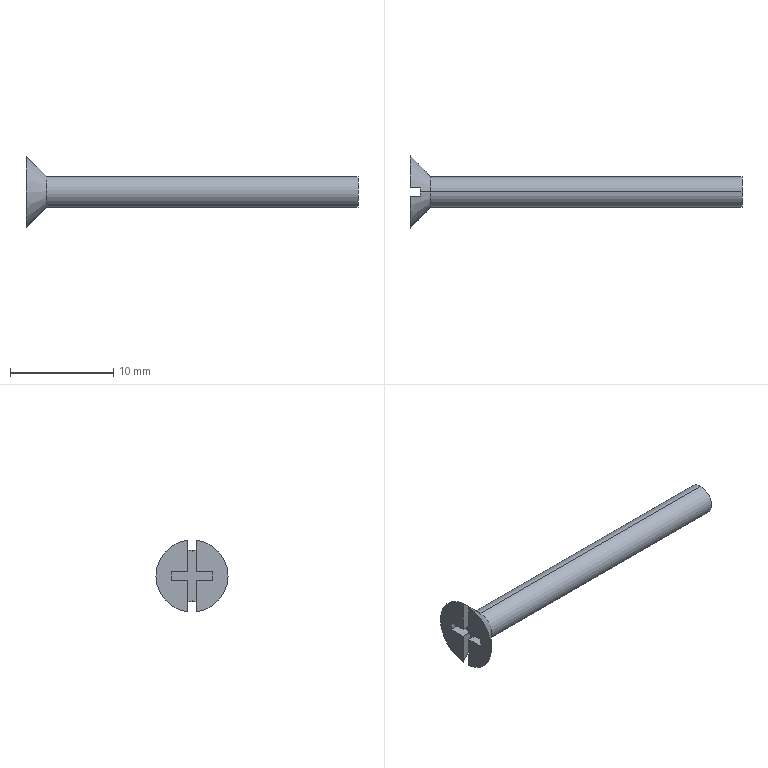Part | STEP file | 4V430C_15_Valve_Screw_L | 1 solid | 18 faces | box 32.2 x 7 x 6.954 mm | volume 247.49 mm3 | plane 14 | cylinder 2 | cone 2 | commonest cylinder face diameters 3 x2
STEP:
#1=CARTESIAN_POINT('',(0.,0.,0.));
#2=DIRECTION('',(0.,0.,1.));
#3=DIRECTION('',(1.,0.,0.));
#4=AXIS2_PLACEMENT_3D('',#1,#2,#3);
#5=CARTESIAN_POINT('',(32.2,0.,1.5));
#6=VERTEX_POINT('',#5);
#7=CARTESIAN_POINT('',(32.2,0.,-1.5));
#8=VERTEX_POINT('',#7);
#9=CARTESIAN_POINT('',(32.2,0.,0.));
#10=DIRECTION('',(-1.,0.,0.));
#11=DIRECTION('',(0.,0.,1.));
#12=AXIS2_PLACEMENT_3D('',#9,#10,#11);
#13=CIRCLE('',#12,1.5);
#14=CARTESIAN_POINT('',(32.2,0.,0.));
#15=DIRECTION('',(-1.,0.,0.));
#16=DIRECTION('',(0.,0.,1.));
#17=AXIS2_PLACEMENT_3D('',#14,#15,#16);
#18=CYLINDRICAL_SURFACE('',#17,1.5);
#19=CARTESIAN_POINT('',(0.,0.));
#20=DIRECTION('',(1.,0.));
#21=VECTOR('',#20,1.);
#22=LINE('',#19,#21);
#23=(GEOMETRIC_REPRESENTATION_CONTEXT(2)PARAMETRIC_REPRESENTATION_CONTEXT()REPRESENTATION_CONTEXT('',''));
#24=DEFINITIONAL_REPRESENTATION('',(#22),#23);
#25=PCURVE('',#18,#24);
#26=CARTESIAN_POINT('',(32.2,1.5,0.));
#27=DIRECTION('',(-1.,0.,0.));
#28=DIRECTION('',(0.,0.,1.));
#29=AXIS2_PLACEMENT_3D('',#26,#27,#28);
#30=PLANE('',#29);
#31=CARTESIAN_POINT('',(0.,-1.5));
#32=DIRECTION('',(1.,0.));
#33=AXIS2_PLACEMENT_2D('',#31,#32);
#34=CIRCLE('',#33,1.5);
#35=(GEOMETRIC_REPRESENTATION_CONTEXT(2)PARAMETRIC_REPRESENTATION_CONTEXT()REPRESENTATION_CONTEXT('',''));
#36=DEFINITIONAL_REPRESENTATION('',(#34),#35);
#37=PCURVE('',#30,#36);
#38=SURFACE_CURVE('',#13,(#25,#37),.PCURVE_S1.);
#39=EDGE_CURVE('',#6,#8,#38,.T.);
#40=ORIENTED_EDGE('',*,*,#39,.T.);
#41=CARTESIAN_POINT('',(2.,0.,-1.5));
#42=VERTEX_POINT('',#41);
#43=CARTESIAN_POINT('',(32.2,0.,-1.5));
#44=DIRECTION('',(-1.,0.,0.));
#45=VECTOR('',#44,1.);
#46=LINE('',#43,#45);
#47=CARTESIAN_POINT('',(3.142,0.));
#48=DIRECTION('',(0.,1.));
#49=VECTOR('',#48,1.);
#50=LINE('',#47,#49);
#51=(GEOMETRIC_REPRESENTATION_CONTEXT(2)PARAMETRIC_REPRESENTATION_CONTEXT()REPRESENTATION_CONTEXT('',''));
#52=DEFINITIONAL_REPRESENTATION('',(#50),#51);
#53=PCURVE('',#18,#52);
#54=CARTESIAN_POINT('',(32.2,0.,0.));
#55=DIRECTION('',(-1.,0.,0.));
#56=DIRECTION('',(0.,0.,1.));
#57=AXIS2_PLACEMENT_3D('',#54,#55,#56);
#58=CYLINDRICAL_SURFACE('',#57,1.5);
#59=CARTESIAN_POINT('',(3.142,0.));
#60=DIRECTION('',(0.,1.));
#61=VECTOR('',#60,1.);
#62=LINE('',#59,#61);
#63=(GEOMETRIC_REPRESENTATION_CONTEXT(2)PARAMETRIC_REPRESENTATION_CONTEXT()REPRESENTATION_CONTEXT('',''));
#64=DEFINITIONAL_REPRESENTATION('',(#62),#63);
#65=PCURVE('',#58,#64);
#66=SURFACE_CURVE('',#46,(#53,#65),.PCURVE_S1.);
#67=EDGE_CURVE('',#8,#42,#66,.T.);
#68=ORIENTED_EDGE('',*,*,#67,.T.);
#69=CARTESIAN_POINT('',(2.,0.,1.5));
#70=VERTEX_POINT('',#69);
#71=CARTESIAN_POINT('',(2.,0.,0.));
#72=DIRECTION('',(-1.,0.,0.));
#73=DIRECTION('',(0.,0.,1.));
#74=AXIS2_PLACEMENT_3D('',#71,#72,#73);
#75=CIRCLE('',#74,1.5);
#76=CARTESIAN_POINT('',(0.,30.2));
#77=DIRECTION('',(1.,0.));
#78=VECTOR('',#77,1.);
#79=LINE('',#76,#78);
#80=(GEOMETRIC_REPRESENTATION_CONTEXT(2)PARAMETRIC_REPRESENTATION_CONTEXT()REPRESENTATION_CONTEXT('',''));
#81=DEFINITIONAL_REPRESENTATION('',(#79),#80);
#82=PCURVE('',#18,#81);
#83=CARTESIAN_POINT('',(2.,0.,0.));
#84=DIRECTION('',(-1.,0.,0.));
#85=DIRECTION('',(0.,0.,1.));
#86=AXIS2_PLACEMENT_3D('',#83,#84,#85);
#87=CONICAL_SURFACE('',#86,1.5,0.7854);
#88=CARTESIAN_POINT('',(0.,0.));
#89=DIRECTION('',(1.,0.));
#90=VECTOR('',#89,1.);
#91=LINE('',#88,#90);
#92=(GEOMETRIC_REPRESENTATION_CONTEXT(2)PARAMETRIC_REPRESENTATION_CONTEXT()REPRESENTATION_CONTEXT('',''));
#93=DEFINITIONAL_REPRESENTATION('',(#91),#92);
#94=PCURVE('',#87,#93);
#95=SURFACE_CURVE('',#75,(#82,#94),.PCURVE_S1.);
#96=EDGE_CURVE('',#70,#42,#95,.T.);
#97=ORIENTED_EDGE('',*,*,#96,.F.);
#98=CARTESIAN_POINT('',(32.2,0.,1.5));
#99=DIRECTION('',(-1.,0.,0.));
#100=VECTOR('',#99,1.);
#101=LINE('',#98,#100);
#102=CARTESIAN_POINT('',(0.,0.));
#103=DIRECTION('',(0.,1.));
#104=VECTOR('',#103,1.);
#105=LINE('',#102,#104);
#106=(GEOMETRIC_REPRESENTATION_CONTEXT(2)PARAMETRIC_REPRESENTATION_CONTEXT()REPRESENTATION_CONTEXT('',''));
#107=DEFINITIONAL_REPRESENTATION('',(#105),#106);
#108=PCURVE('',#18,#107);
#109=CARTESIAN_POINT('',(6.283,0.));
#110=DIRECTION('',(0.,1.));
#111=VECTOR('',#110,1.);
#112=LINE('',#109,#111);
#113=(GEOMETRIC_REPRESENTATION_CONTEXT(2)PARAMETRIC_REPRESENTATION_CONTEXT()REPRESENTATION_CONTEXT('',''));
#114=DEFINITIONAL_REPRESENTATION('',(#112),#113);
#115=PCURVE('',#58,#114);
#116=SURFACE_CURVE('',#101,(#108,#115),.PCURVE_S1.);
#117=EDGE_CURVE('',#6,#70,#116,.T.);
#118=ORIENTED_EDGE('',*,*,#117,.F.);
#119=EDGE_LOOP('',(#40,#68,#97,#118));
#120=FACE_BOUND('',#119,.T.);
#121=ADVANCED_FACE('',(#120),#18,.T.);
#122=ORIENTED_EDGE('',*,*,#96,.T.);
#123=CARTESIAN_POINT('',(1.,0.,-2.5));
#124=VERTEX_POINT('',#123);
#125=CARTESIAN_POINT('',(2.,0.,-1.5));
#126=DIRECTION('',(-0.7071,0.,-0.7071));
#127=VECTOR('',#126,1.);
#128=LINE('',#125,#127);
#129=CARTESIAN_POINT('',(3.142,0.));
#130=DIRECTION('',(0.,1.));
#131=VECTOR('',#130,1.);
#132=LINE('',#129,#131);
#133=(GEOMETRIC_REPRESENTATION_CONTEXT(2)PARAMETRIC_REPRESENTATION_CONTEXT()REPRESENTATION_CONTEXT('',''));
#134=DEFINITIONAL_REPRESENTATION('',(#132),#133);
#135=PCURVE('',#87,#134);
#136=CARTESIAN_POINT('',(2.,0.,0.));
#137=DIRECTION('',(-1.,0.,0.));
#138=DIRECTION('',(0.,0.,1.));
#139=AXIS2_PLACEMENT_3D('',#136,#137,#138);
#140=CONICAL_SURFACE('',#139,1.5,0.7854);
#141=CARTESIAN_POINT('',(3.142,0.));
#142=DIRECTION('',(0.,1.));
#143=VECTOR('',#142,1.);
#144=LINE('',#141,#143);
#145=(GEOMETRIC_REPRESENTATION_CONTEXT(2)PARAMETRIC_REPRESENTATION_CONTEXT()REPRESENTATION_CONTEXT('',''));
#146=DEFINITIONAL_REPRESENTATION('',(#144),#145);
#147=PCURVE('',#140,#146);
#148=SURFACE_CURVE('',#128,(#135,#147),.PCURVE_S1.);
#149=EDGE_CURVE('',#42,#124,#148,.T.);
#150=ORIENTED_EDGE('',*,*,#149,.T.);
#151=CARTESIAN_POINT('',(1.,0.4,-2.468));
#152=VERTEX_POINT('',#151);
#153=CARTESIAN_POINT('',(1.,0.,0.));
#154=DIRECTION('',(1.,0.,0.));
#155=DIRECTION('',(0.,0.,-1.));
#156=AXIS2_PLACEMENT_3D('',#153,#154,#155);
#157=CIRCLE('',#156,2.5);
#158=CARTESIAN_POINT('',(3.142,1.));
#159=DIRECTION('',(-1.,0.));
#160=VECTOR('',#159,1.);
#161=LINE('',#158,#160);
#162=(GEOMETRIC_REPRESENTATION_CONTEXT(2)PARAMETRIC_REPRESENTATION_CONTEXT()REPRESENTATION_CONTEXT('',''));
#163=DEFINITIONAL_REPRESENTATION('',(#161),#162);
#164=PCURVE('',#87,#163);
#165=CARTESIAN_POINT('',(1.,0.4,4.));
#166=DIRECTION('',(1.,0.,0.));
#167=DIRECTION('',(0.,0.,-1.));
#168=AXIS2_PLACEMENT_3D('',#165,#166,#167);
#169=PLANE('',#168);
#170=CARTESIAN_POINT('',(4.,-0.4));
#171=DIRECTION('',(1.,0.));
#172=AXIS2_PLACEMENT_2D('',#170,#171);
#173=CIRCLE('',#172,2.5);
#174=(GEOMETRIC_REPRESENTATION_CONTEXT(2)PARAMETRIC_REPRESENTATION_CONTEXT()REPRESENTATION_CONTEXT('',''));
#175=DEFINITIONAL_REPRESENTATION('',(#173),#174);
#176=PCURVE('',#169,#175);
#177=SURFACE_CURVE('',#157,(#164,#176),.PCURVE_S1.);
#178=EDGE_CURVE('',#124,#152,#177,.T.);
#179=ORIENTED_EDGE('',*,*,#178,.T.);
#180=CARTESIAN_POINT('',(0.,0.4,-3.477));
#181=VERTEX_POINT('',#180);
#182=CARTESIAN_POINT('',(0.,0.4,-3.477));
#183=CARTESIAN_POINT('',(0.3338,0.4,-3.141));
#184=CARTESIAN_POINT('',(0.6673,0.4,-2.805));
#185=CARTESIAN_POINT('',(1.,0.4,-2.468));
#186=B_SPLINE_CURVE_WITH_KNOTS('',3,(#182,#183,#184,#185),.UNSPECIFIED.,.F.,.F.,(4,4),(0.002985,0.004406),.PIECEWISE_BEZIER_KNOTS.);
#187=CARTESIAN_POINT('',(3.027,2.));
#188=CARTESIAN_POINT('',(3.027,1.985));
#189=CARTESIAN_POINT('',(3.026,1.954));
#190=CARTESIAN_POINT('',(3.024,1.909));
#191=CARTESIAN_POINT('',(3.022,1.863));
#192=CARTESIAN_POINT('',(3.021,1.818));
#193=CARTESIAN_POINT('',(3.019,1.772));
#194=CARTESIAN_POINT('',(3.017,1.727));
#195=CARTESIAN_POINT('',(3.016,1.681));
#196=CARTESIAN_POINT('',(3.014,1.636));
#197=CARTESIAN_POINT('',(3.012,1.591));
#198=CARTESIAN_POINT('',(3.01,1.545));
#199=CARTESIAN_POINT('',(3.008,1.5));
#200=CARTESIAN_POINT('',(3.006,1.454));
#201=CARTESIAN_POINT('',(3.004,1.409));
#202=CARTESIAN_POINT('',(3.001,1.363));
#203=CARTESIAN_POINT('',(2.999,1.318));
#204=CARTESIAN_POINT('',(2.997,1.272));
#205=CARTESIAN_POINT('',(2.994,1.227));
#206=CARTESIAN_POINT('',(2.992,1.182));
#207=CARTESIAN_POINT('',(2.989,1.136));
#208=CARTESIAN_POINT('',(2.987,1.091));
#209=CARTESIAN_POINT('',(2.984,1.045));
#210=CARTESIAN_POINT('',(2.982,1.015));
#211=CARTESIAN_POINT('',(2.981,1.));
#212=B_SPLINE_CURVE_WITH_KNOTS('',3,(#187,#188,#189,#190,#191,#192,#193,#194,#195,#196,#197,#198,#199,#200,#201,#202,#203,#204,#205,#206,#207,#208,#209,#210,#211),.UNSPECIFIED.,.F.,.F.,(4,1,1,1,1,1,1,1,1,1,1,1,1,1,1,1,1,1,1,1,1,1,4),(0.002985,0.00305,0.003115,0.003179,0.003244,0.003308,0.003373,0.003437,0.003502,0.003567,0.003631,0.003696,0.00376,0.003825,0.003889,0.003954,0.004019,0.004083,0.004148,0.004212,0.004277,0.004342,0.004406),.QUASI_UNIFORM_KNOTS.);
#213=(GEOMETRIC_REPRESENTATION_CONTEXT(2)PARAMETRIC_REPRESENTATION_CONTEXT()REPRESENTATION_CONTEXT('',''));
#214=DEFINITIONAL_REPRESENTATION('',(#212),#213);
#215=PCURVE('',#87,#214);
#216=CARTESIAN_POINT('',(1.,0.4,-4.));
#217=DIRECTION('',(0.,-1.,0.));
#218=DIRECTION('',(0.,0.,-1.));
#219=AXIS2_PLACEMENT_3D('',#216,#217,#218);
#220=PLANE('',#219);
#221=CARTESIAN_POINT('',(-0.5229,-1.));
#222=CARTESIAN_POINT('',(-0.8589,-0.6662));
#223=CARTESIAN_POINT('',(-1.195,-0.3327));
#224=CARTESIAN_POINT('',(-1.532,0.));
#225=B_SPLINE_CURVE_WITH_KNOTS('',3,(#221,#222,#223,#224),.UNSPECIFIED.,.F.,.F.,(4,4),(0.002985,0.004406),.PIECEWISE_BEZIER_KNOTS.);
#226=(GEOMETRIC_REPRESENTATION_CONTEXT(2)PARAMETRIC_REPRESENTATION_CONTEXT()REPRESENTATION_CONTEXT('',''));
#227=DEFINITIONAL_REPRESENTATION('',(#225),#226);
#228=PCURVE('',#220,#227);
#229=SURFACE_CURVE('',#186,(#215,#228),.PCURVE_S1.);
#230=EDGE_CURVE('',#181,#152,#229,.T.);
#231=ORIENTED_EDGE('',*,*,#230,.F.);
#232=CARTESIAN_POINT('',(0.,0.4,3.477));
#233=VERTEX_POINT('',#232);
#234=CARTESIAN_POINT('',(0.,0.,0.));
#235=DIRECTION('',(-1.,0.,0.));
#236=DIRECTION('',(0.,0.,1.));
#237=AXIS2_PLACEMENT_3D('',#234,#235,#236);
#238=CIRCLE('',#237,3.5);
#239=CARTESIAN_POINT('',(0.,2.));
#240=DIRECTION('',(1.,0.));
#241=VECTOR('',#240,1.);
#242=LINE('',#239,#241);
#243=(GEOMETRIC_REPRESENTATION_CONTEXT(2)PARAMETRIC_REPRESENTATION_CONTEXT()REPRESENTATION_CONTEXT('',''));
#244=DEFINITIONAL_REPRESENTATION('',(#242),#243);
#245=PCURVE('',#87,#244);
#246=CARTESIAN_POINT('',(0.,0.,0.));
#247=DIRECTION('',(1.,0.,0.));
#248=DIRECTION('',(0.,0.,-1.));
#249=AXIS2_PLACEMENT_3D('',#246,#247,#248);
#250=PLANE('',#249);
#251=CARTESIAN_POINT('',(-3.5,0.));
#252=CARTESIAN_POINT('',(-3.5,6.062));
#253=CARTESIAN_POINT('',(1.75,3.031));
#254=CARTESIAN_POINT('',(7.,0.));
#255=CARTESIAN_POINT('',(1.75,-3.031));
#256=CARTESIAN_POINT('',(-3.5,-6.062));
#257=CARTESIAN_POINT('',(-3.5,0.));
#258=(BOUNDED_CURVE()B_SPLINE_CURVE(2,(#251,#252,#253,#254,#255,#256,#257),.UNSPECIFIED.,.T.,.F.)B_SPLINE_CURVE_WITH_KNOTS((1,2,2,2,2,1),(-2.094,0.,2.094,4.189,6.283,8.378),.UNSPECIFIED.)CURVE()GEOMETRIC_REPRESENTATION_ITEM()RATIONAL_B_SPLINE_CURVE((1.,0.5,1.,0.5,1.,0.5,1.))REPRESENTATION_ITEM(''));
#259=(GEOMETRIC_REPRESENTATION_CONTEXT(2)PARAMETRIC_REPRESENTATION_CONTEXT()REPRESENTATION_CONTEXT('',''));
#260=DEFINITIONAL_REPRESENTATION('',(#258),#259);
#261=PCURVE('',#250,#260);
#262=SURFACE_CURVE('',#238,(#245,#261),.PCURVE_S1.);
#263=EDGE_CURVE('',#233,#181,#262,.T.);
#264=ORIENTED_EDGE('',*,*,#263,.F.);
#265=CARTESIAN_POINT('',(1.,0.4,2.468));
#266=VERTEX_POINT('',#265);
#267=CARTESIAN_POINT('',(1.,0.4,2.468));
#268=CARTESIAN_POINT('',(0.6673,0.4,2.805));
#269=CARTESIAN_POINT('',(0.3338,0.4,3.141));
#270=CARTESIAN_POINT('',(0.,0.4,3.477));
#271=B_SPLINE_CURVE_WITH_KNOTS('',3,(#267,#268,#269,#270),.UNSPECIFIED.,.F.,.F.,(4,4),(0.002885,0.004305),.PIECEWISE_BEZIER_KNOTS.);
#272=CARTESIAN_POINT('',(0.1607,1.));
#273=CARTESIAN_POINT('',(0.1597,1.015));
#274=CARTESIAN_POINT('',(0.1578,1.045));
#275=CARTESIAN_POINT('',(0.155,1.091));
#276=CARTESIAN_POINT('',(0.1523,1.136));
#277=CARTESIAN_POINT('',(0.1497,1.182));
#278=CARTESIAN_POINT('',(0.1472,1.227));
#279=CARTESIAN_POINT('',(0.1448,1.272));
#280=CARTESIAN_POINT('',(0.1424,1.318));
#281=CARTESIAN_POINT('',(0.1401,1.363));
#282=CARTESIAN_POINT('',(0.1379,1.409));
#283=CARTESIAN_POINT('',(0.1358,1.454));
#284=CARTESIAN_POINT('',(0.1337,1.5));
#285=CARTESIAN_POINT('',(0.1317,1.545));
#286=CARTESIAN_POINT('',(0.1298,1.591));
#287=CARTESIAN_POINT('',(0.1279,1.636));
#288=CARTESIAN_POINT('',(0.1261,1.681));
#289=CARTESIAN_POINT('',(0.1243,1.727));
#290=CARTESIAN_POINT('',(0.1225,1.772));
#291=CARTESIAN_POINT('',(0.1208,1.818));
#292=CARTESIAN_POINT('',(0.1192,1.863));
#293=CARTESIAN_POINT('',(0.1176,1.909));
#294=CARTESIAN_POINT('',(0.116,1.954));
#295=CARTESIAN_POINT('',(0.115,1.985));
#296=CARTESIAN_POINT('',(0.1145,2.));
#297=B_SPLINE_CURVE_WITH_KNOTS('',3,(#272,#273,#274,#275,#276,#277,#278,#279,#280,#281,#282,#283,#284,#285,#286,#287,#288,#289,#290,#291,#292,#293,#294,#295,#296),.UNSPECIFIED.,.F.,.F.,(4,1,1,1,1,1,1,1,1,1,1,1,1,1,1,1,1,1,1,1,1,1,4),(0.002885,0.002949,0.003014,0.003078,0.003143,0.003207,0.003272,0.003337,0.003401,0.003466,0.00353,0.003595,0.003659,0.003724,0.003788,0.003853,0.003917,0.003982,0.004046,0.004111,0.004175,0.00424,0.004305),.QUASI_UNIFORM_KNOTS.);
#298=(GEOMETRIC_REPRESENTATION_CONTEXT(2)PARAMETRIC_REPRESENTATION_CONTEXT()REPRESENTATION_CONTEXT('',''));
#299=DEFINITIONAL_REPRESENTATION('',(#297),#298);
#300=PCURVE('',#87,#299);
#301=CARTESIAN_POINT('',(1.,0.4,0.4));
#302=DIRECTION('',(0.,-1.,0.));
#303=DIRECTION('',(0.,0.,-1.));
#304=AXIS2_PLACEMENT_3D('',#301,#302,#303);
#305=PLANE('',#304);
#306=CARTESIAN_POINT('',(-2.068,0.));
#307=CARTESIAN_POINT('',(-2.405,-0.3327));
#308=CARTESIAN_POINT('',(-2.741,-0.6662));
#309=CARTESIAN_POINT('',(-3.077,-1.));
#310=B_SPLINE_CURVE_WITH_KNOTS('',3,(#306,#307,#308,#309),.UNSPECIFIED.,.F.,.F.,(4,4),(0.002885,0.004305),.PIECEWISE_BEZIER_KNOTS.);
#311=(GEOMETRIC_REPRESENTATION_CONTEXT(2)PARAMETRIC_REPRESENTATION_CONTEXT()REPRESENTATION_CONTEXT('',''));
#312=DEFINITIONAL_REPRESENTATION('',(#310),#311);
#313=PCURVE('',#305,#312);
#314=SURFACE_CURVE('',#271,(#300,#313),.PCURVE_S1.);
#315=EDGE_CURVE('',#266,#233,#314,.T.);
#316=ORIENTED_EDGE('',*,*,#315,.F.);
#317=CARTESIAN_POINT('',(1.,0.,2.5));
#318=VERTEX_POINT('',#317);
#319=CARTESIAN_POINT('',(1.,0.,0.));
#320=DIRECTION('',(1.,0.,0.));
#321=DIRECTION('',(0.,0.,-1.));
#322=AXIS2_PLACEMENT_3D('',#319,#320,#321);
#323=CIRCLE('',#322,2.5);
#324=CARTESIAN_POINT('',(3.142,1.));
#325=DIRECTION('',(-1.,0.));
#326=VECTOR('',#325,1.);
#327=LINE('',#324,#326);
#328=(GEOMETRIC_REPRESENTATION_CONTEXT(2)PARAMETRIC_REPRESENTATION_CONTEXT()REPRESENTATION_CONTEXT('',''));
#329=DEFINITIONAL_REPRESENTATION('',(#327),#328);
#330=PCURVE('',#87,#329);
#331=CARTESIAN_POINT('',(4.,-0.4));
#332=DIRECTION('',(1.,0.));
#333=AXIS2_PLACEMENT_2D('',#331,#332);
#334=CIRCLE('',#333,2.5);
#335=(GEOMETRIC_REPRESENTATION_CONTEXT(2)PARAMETRIC_REPRESENTATION_CONTEXT()REPRESENTATION_CONTEXT('',''));
#336=DEFINITIONAL_REPRESENTATION('',(#334),#335);
#337=PCURVE('',#169,#336);
#338=SURFACE_CURVE('',#323,(#330,#337),.PCURVE_S1.);
#339=EDGE_CURVE('',#266,#318,#338,.T.);
#340=ORIENTED_EDGE('',*,*,#339,.T.);
#341=CARTESIAN_POINT('',(2.,0.,1.5));
#342=DIRECTION('',(-0.7071,0.,0.7071));
#343=VECTOR('',#342,1.);
#344=LINE('',#341,#343);
#345=CARTESIAN_POINT('',(0.,0.));
#346=DIRECTION('',(0.,1.));
#347=VECTOR('',#346,1.);
#348=LINE('',#345,#347);
#349=(GEOMETRIC_REPRESENTATION_CONTEXT(2)PARAMETRIC_REPRESENTATION_CONTEXT()REPRESENTATION_CONTEXT('',''));
#350=DEFINITIONAL_REPRESENTATION('',(#348),#349);
#351=PCURVE('',#87,#350);
#352=CARTESIAN_POINT('',(6.283,0.));
#353=DIRECTION('',(0.,1.));
#354=VECTOR('',#353,1.);
#355=LINE('',#352,#354);
#356=(GEOMETRIC_REPRESENTATION_CONTEXT(2)PARAMETRIC_REPRESENTATION_CONTEXT()REPRESENTATION_CONTEXT('',''));
#357=DEFINITIONAL_REPRESENTATION('',(#355),#356);
#358=PCURVE('',#140,#357);
#359=SURFACE_CURVE('',#344,(#351,#358),.PCURVE_S1.);
#360=EDGE_CURVE('',#70,#318,#359,.T.);
#361=ORIENTED_EDGE('',*,*,#360,.F.);
#362=EDGE_LOOP('',(#122,#150,#179,#231,#264,#316,#340,#361));
#363=FACE_BOUND('',#362,.T.);
#364=ADVANCED_FACE('',(#363),#87,.T.);
#365=CARTESIAN_POINT('',(0.,-0.4,3.477));
#366=VERTEX_POINT('',#365);
#367=CARTESIAN_POINT('',(0.,-0.4,0.4));
#368=VERTEX_POINT('',#367);
#369=CARTESIAN_POINT('',(0.,-0.4,4.));
#370=DIRECTION('',(0.,0.,-1.));
#371=VECTOR('',#370,1.);
#372=LINE('',#369,#371);
#373=CARTESIAN_POINT('',(0.,0.,0.));
#374=DIRECTION('',(1.,0.,0.));
#375=DIRECTION('',(0.,0.,-1.));
#376=AXIS2_PLACEMENT_3D('',#373,#374,#375);
#377=PLANE('',#376);
#378=CARTESIAN_POINT('',(-4.,-0.4));
#379=DIRECTION('',(1.,0.));
#380=VECTOR('',#379,1.);
#381=LINE('',#378,#380);
#382=(GEOMETRIC_REPRESENTATION_CONTEXT(2)PARAMETRIC_REPRESENTATION_CONTEXT()REPRESENTATION_CONTEXT('',''));
#383=DEFINITIONAL_REPRESENTATION('',(#381),#382);
#384=PCURVE('',#377,#383);
#385=CARTESIAN_POINT('',(1.,-0.4,4.));
#386=DIRECTION('',(0.,1.,0.));
#387=DIRECTION('',(0.,0.,1.));
#388=AXIS2_PLACEMENT_3D('',#385,#386,#387);
#389=PLANE('',#388);
#390=CARTESIAN_POINT('',(0.,-1.));
#391=DIRECTION('',(-1.,0.));
#392=VECTOR('',#391,1.);
#393=LINE('',#390,#392);
#394=(GEOMETRIC_REPRESENTATION_CONTEXT(2)PARAMETRIC_REPRESENTATION_CONTEXT()REPRESENTATION_CONTEXT('',''));
#395=DEFINITIONAL_REPRESENTATION('',(#393),#394);
#396=PCURVE('',#389,#395);
#397=SURFACE_CURVE('',#372,(#384,#396),.PCURVE_S1.);
#398=EDGE_CURVE('',#366,#368,#397,.T.);
#399=ORIENTED_EDGE('',*,*,#398,.T.);
#400=CARTESIAN_POINT('',(0.,-2.,0.4));
#401=VERTEX_POINT('',#400);
#402=CARTESIAN_POINT('',(0.,-0.4,0.4));
#403=DIRECTION('',(0.,-1.,0.));
#404=VECTOR('',#403,1.);
#405=LINE('',#402,#404);
#406=CARTESIAN_POINT('',(-0.4,-0.4));
#407=DIRECTION('',(0.,-1.));
#408=VECTOR('',#407,1.);
#409=LINE('',#406,#408);
#410=(GEOMETRIC_REPRESENTATION_CONTEXT(2)PARAMETRIC_REPRESENTATION_CONTEXT()REPRESENTATION_CONTEXT('',''));
#411=DEFINITIONAL_REPRESENTATION('',(#409),#410);
#412=PCURVE('',#377,#411);
#413=CARTESIAN_POINT('',(1.,-0.4,0.4));
#414=DIRECTION('',(0.,0.,-1.));
#415=DIRECTION('',(0.,1.,0.));
#416=AXIS2_PLACEMENT_3D('',#413,#414,#415);
#417=PLANE('',#416);
#418=CARTESIAN_POINT('',(0.,-1.));
#419=DIRECTION('',(-1.,0.));
#420=VECTOR('',#419,1.);
#421=LINE('',#418,#420);
#422=(GEOMETRIC_REPRESENTATION_CONTEXT(2)PARAMETRIC_REPRESENTATION_CONTEXT()REPRESENTATION_CONTEXT('',''));
#423=DEFINITIONAL_REPRESENTATION('',(#421),#422);
#424=PCURVE('',#417,#423);
#425=SURFACE_CURVE('',#405,(#412,#424),.PCURVE_S1.);
#426=EDGE_CURVE('',#368,#401,#425,.T.);
#427=ORIENTED_EDGE('',*,*,#426,.T.);
#428=CARTESIAN_POINT('',(0.,-2.,-0.4));
#429=VERTEX_POINT('',#428);
#430=CARTESIAN_POINT('',(0.,-2.,0.4));
#431=DIRECTION('',(0.,0.,-1.));
#432=VECTOR('',#431,1.);
#433=LINE('',#430,#432);
#434=CARTESIAN_POINT('',(-0.4,-2.));
#435=DIRECTION('',(1.,0.));
#436=VECTOR('',#435,1.);
#437=LINE('',#434,#436);
#438=(GEOMETRIC_REPRESENTATION_CONTEXT(2)PARAMETRIC_REPRESENTATION_CONTEXT()REPRESENTATION_CONTEXT('',''));
#439=DEFINITIONAL_REPRESENTATION('',(#437),#438);
#440=PCURVE('',#377,#439);
#441=CARTESIAN_POINT('',(1.,-2.,0.4));
#442=DIRECTION('',(0.,1.,0.));
#443=DIRECTION('',(0.,0.,1.));
#444=AXIS2_PLACEMENT_3D('',#441,#442,#443);
#445=PLANE('',#444);
#446=CARTESIAN_POINT('',(0.,-1.));
#447=DIRECTION('',(-1.,0.));
#448=VECTOR('',#447,1.);
#449=LINE('',#446,#448);
#450=(GEOMETRIC_REPRESENTATION_CONTEXT(2)PARAMETRIC_REPRESENTATION_CONTEXT()REPRESENTATION_CONTEXT('',''));
#451=DEFINITIONAL_REPRESENTATION('',(#449),#450);
#452=PCURVE('',#445,#451);
#453=SURFACE_CURVE('',#433,(#440,#452),.PCURVE_S1.);
#454=EDGE_CURVE('',#401,#429,#453,.T.);
#455=ORIENTED_EDGE('',*,*,#454,.T.);
#456=CARTESIAN_POINT('',(0.,-0.4,-0.4));
#457=VERTEX_POINT('',#456);
#458=CARTESIAN_POINT('',(0.,-2.,-0.4));
#459=DIRECTION('',(0.,1.,0.));
#460=VECTOR('',#459,1.);
#461=LINE('',#458,#460);
#462=CARTESIAN_POINT('',(0.4,-2.));
#463=DIRECTION('',(0.,1.));
#464=VECTOR('',#463,1.);
#465=LINE('',#462,#464);
#466=(GEOMETRIC_REPRESENTATION_CONTEXT(2)PARAMETRIC_REPRESENTATION_CONTEXT()REPRESENTATION_CONTEXT('',''));
#467=DEFINITIONAL_REPRESENTATION('',(#465),#466);
#468=PCURVE('',#377,#467);
#469=CARTESIAN_POINT('',(1.,-2.,-0.4));
#470=DIRECTION('',(0.,0.,1.));
#471=DIRECTION('',(1.,0.,0.));
#472=AXIS2_PLACEMENT_3D('',#469,#470,#471);
#473=PLANE('',#472);
#474=CARTESIAN_POINT('',(-1.,0.));
#475=DIRECTION('',(0.,1.));
#476=VECTOR('',#475,1.);
#477=LINE('',#474,#476);
#478=(GEOMETRIC_REPRESENTATION_CONTEXT(2)PARAMETRIC_REPRESENTATION_CONTEXT()REPRESENTATION_CONTEXT('',''));
#479=DEFINITIONAL_REPRESENTATION('',(#477),#478);
#480=PCURVE('',#473,#479);
#481=SURFACE_CURVE('',#461,(#468,#480),.PCURVE_S1.);
#482=EDGE_CURVE('',#429,#457,#481,.T.);
#483=ORIENTED_EDGE('',*,*,#482,.T.);
#484=CARTESIAN_POINT('',(0.,-0.4,-3.477));
#485=VERTEX_POINT('',#484);
#486=CARTESIAN_POINT('',(0.,-0.4,-0.4));
#487=DIRECTION('',(0.,0.,-1.));
#488=VECTOR('',#487,1.);
#489=LINE('',#486,#488);
#490=CARTESIAN_POINT('',(0.4,-0.4));
#491=DIRECTION('',(1.,0.));
#492=VECTOR('',#491,1.);
#493=LINE('',#490,#492);
#494=(GEOMETRIC_REPRESENTATION_CONTEXT(2)PARAMETRIC_REPRESENTATION_CONTEXT()REPRESENTATION_CONTEXT('',''));
#495=DEFINITIONAL_REPRESENTATION('',(#493),#494);
#496=PCURVE('',#377,#495);
#497=CARTESIAN_POINT('',(1.,-0.4,-0.4));
#498=DIRECTION('',(0.,1.,0.));
#499=DIRECTION('',(0.,0.,1.));
#500=AXIS2_PLACEMENT_3D('',#497,#498,#499);
#501=PLANE('',#500);
#502=CARTESIAN_POINT('',(0.,-1.));
#503=DIRECTION('',(-1.,0.));
#504=VECTOR('',#503,1.);
#505=LINE('',#502,#504);
#506=(GEOMETRIC_REPRESENTATION_CONTEXT(2)PARAMETRIC_REPRESENTATION_CONTEXT()REPRESENTATION_CONTEXT('',''));
#507=DEFINITIONAL_REPRESENTATION('',(#505),#506);
#508=PCURVE('',#501,#507);
#509=SURFACE_CURVE('',#489,(#496,#508),.PCURVE_S1.);
#510=EDGE_CURVE('',#457,#485,#509,.T.);
#511=ORIENTED_EDGE('',*,*,#510,.T.);
#512=CARTESIAN_POINT('',(0.,0.,0.));
#513=DIRECTION('',(-1.,0.,0.));
#514=DIRECTION('',(0.,0.,1.));
#515=AXIS2_PLACEMENT_3D('',#512,#513,#514);
#516=CIRCLE('',#515,3.5);
#517=CARTESIAN_POINT('',(-3.5,0.));
#518=CARTESIAN_POINT('',(-3.5,6.062));
#519=CARTESIAN_POINT('',(1.75,3.031));
#520=CARTESIAN_POINT('',(7.,0.));
#521=CARTESIAN_POINT('',(1.75,-3.031));
#522=CARTESIAN_POINT('',(-3.5,-6.062));
#523=CARTESIAN_POINT('',(-3.5,0.));
#524=(BOUNDED_CURVE()B_SPLINE_CURVE(2,(#517,#518,#519,#520,#521,#522,#523),.UNSPECIFIED.,.T.,.F.)B_SPLINE_CURVE_WITH_KNOTS((1,2,2,2,2,1),(-2.094,0.,2.094,4.189,6.283,8.378),.UNSPECIFIED.)CURVE()GEOMETRIC_REPRESENTATION_ITEM()RATIONAL_B_SPLINE_CURVE((1.,0.5,1.,0.5,1.,0.5,1.))REPRESENTATION_ITEM(''));
#525=(GEOMETRIC_REPRESENTATION_CONTEXT(2)PARAMETRIC_REPRESENTATION_CONTEXT()REPRESENTATION_CONTEXT('',''));
#526=DEFINITIONAL_REPRESENTATION('',(#524),#525);
#527=PCURVE('',#377,#526);
#528=CARTESIAN_POINT('',(0.,2.));
#529=DIRECTION('',(1.,0.));
#530=VECTOR('',#529,1.);
#531=LINE('',#528,#530);
#532=(GEOMETRIC_REPRESENTATION_CONTEXT(2)PARAMETRIC_REPRESENTATION_CONTEXT()REPRESENTATION_CONTEXT('',''));
#533=DEFINITIONAL_REPRESENTATION('',(#531),#532);
#534=PCURVE('',#140,#533);
#535=SURFACE_CURVE('',#516,(#527,#534),.PCURVE_S1.);
#536=EDGE_CURVE('',#485,#366,#535,.T.);
#537=ORIENTED_EDGE('',*,*,#536,.T.);
#538=EDGE_LOOP('',(#399,#427,#455,#483,#511,#537));
#539=FACE_BOUND('',#538,.T.);
#540=ADVANCED_FACE('',(#539),#377,.F.);
#541=CARTESIAN_POINT('',(0.,0.4,0.4));
#542=VERTEX_POINT('',#541);
#543=CARTESIAN_POINT('',(0.,0.4,0.4));
#544=DIRECTION('',(0.,0.,1.));
#545=VECTOR('',#544,1.);
#546=LINE('',#543,#545);
#547=CARTESIAN_POINT('',(-0.4,0.4));
#548=DIRECTION('',(-1.,0.));
#549=VECTOR('',#548,1.);
#550=LINE('',#547,#549);
#551=(GEOMETRIC_REPRESENTATION_CONTEXT(2)PARAMETRIC_REPRESENTATION_CONTEXT()REPRESENTATION_CONTEXT('',''));
#552=DEFINITIONAL_REPRESENTATION('',(#550),#551);
#553=PCURVE('',#250,#552);
#554=CARTESIAN_POINT('',(0.,-1.));
#555=DIRECTION('',(-1.,0.));
#556=VECTOR('',#555,1.);
#557=LINE('',#554,#556);
#558=(GEOMETRIC_REPRESENTATION_CONTEXT(2)PARAMETRIC_REPRESENTATION_CONTEXT()REPRESENTATION_CONTEXT('',''));
#559=DEFINITIONAL_REPRESENTATION('',(#557),#558);
#560=PCURVE('',#305,#559);
#561=SURFACE_CURVE('',#546,(#553,#560),.PCURVE_S1.);
#562=EDGE_CURVE('',#542,#233,#561,.T.);
#563=ORIENTED_EDGE('',*,*,#562,.T.);
#564=ORIENTED_EDGE('',*,*,#263,.T.);
#565=CARTESIAN_POINT('',(0.,0.4,-0.4));
#566=VERTEX_POINT('',#565);
#567=CARTESIAN_POINT('',(0.,0.4,-4.));
#568=DIRECTION('',(0.,0.,1.));
#569=VECTOR('',#568,1.);
#570=LINE('',#567,#569);
#571=CARTESIAN_POINT('',(4.,0.4));
#572=DIRECTION('',(-1.,0.));
#573=VECTOR('',#572,1.);
#574=LINE('',#571,#573);
#575=(GEOMETRIC_REPRESENTATION_CONTEXT(2)PARAMETRIC_REPRESENTATION_CONTEXT()REPRESENTATION_CONTEXT('',''));
#576=DEFINITIONAL_REPRESENTATION('',(#574),#575);
#577=PCURVE('',#250,#576);
#578=CARTESIAN_POINT('',(0.,-1.));
#579=DIRECTION('',(-1.,0.));
#580=VECTOR('',#579,1.);
#581=LINE('',#578,#580);
#582=(GEOMETRIC_REPRESENTATION_CONTEXT(2)PARAMETRIC_REPRESENTATION_CONTEXT()REPRESENTATION_CONTEXT('',''));
#583=DEFINITIONAL_REPRESENTATION('',(#581),#582);
#584=PCURVE('',#220,#583);
#585=SURFACE_CURVE('',#570,(#577,#584),.PCURVE_S1.);
#586=EDGE_CURVE('',#181,#566,#585,.T.);
#587=ORIENTED_EDGE('',*,*,#586,.T.);
#588=CARTESIAN_POINT('',(0.,2.,-0.4));
#589=VERTEX_POINT('',#588);
#590=CARTESIAN_POINT('',(0.,0.4,-0.4));
#591=DIRECTION('',(0.,1.,0.));
#592=VECTOR('',#591,1.);
#593=LINE('',#590,#592);
#594=CARTESIAN_POINT('',(0.4,0.4));
#595=DIRECTION('',(0.,1.));
#596=VECTOR('',#595,1.);
#597=LINE('',#594,#596);
#598=(GEOMETRIC_REPRESENTATION_CONTEXT(2)PARAMETRIC_REPRESENTATION_CONTEXT()REPRESENTATION_CONTEXT('',''));
#599=DEFINITIONAL_REPRESENTATION('',(#597),#598);
#600=PCURVE('',#250,#599);
#601=CARTESIAN_POINT('',(1.,0.4,-0.4));
#602=DIRECTION('',(0.,0.,1.));
#603=DIRECTION('',(0.,-1.,0.));
#604=AXIS2_PLACEMENT_3D('',#601,#602,#603);
#605=PLANE('',#604);
#606=CARTESIAN_POINT('',(0.,-1.));
#607=DIRECTION('',(-1.,0.));
#608=VECTOR('',#607,1.);
#609=LINE('',#606,#608);
#610=(GEOMETRIC_REPRESENTATION_CONTEXT(2)PARAMETRIC_REPRESENTATION_CONTEXT()REPRESENTATION_CONTEXT('',''));
#611=DEFINITIONAL_REPRESENTATION('',(#609),#610);
#612=PCURVE('',#605,#611);
#613=SURFACE_CURVE('',#593,(#600,#612),.PCURVE_S1.);
#614=EDGE_CURVE('',#566,#589,#613,.T.);
#615=ORIENTED_EDGE('',*,*,#614,.T.);
#616=CARTESIAN_POINT('',(0.,2.,0.4));
#617=VERTEX_POINT('',#616);
#618=CARTESIAN_POINT('',(0.,2.,-0.4));
#619=DIRECTION('',(0.,0.,1.));
#620=VECTOR('',#619,1.);
#621=LINE('',#618,#620);
#622=CARTESIAN_POINT('',(0.4,2.));
#623=DIRECTION('',(-1.,0.));
#624=VECTOR('',#623,1.);
#625=LINE('',#622,#624);
#626=(GEOMETRIC_REPRESENTATION_CONTEXT(2)PARAMETRIC_REPRESENTATION_CONTEXT()REPRESENTATION_CONTEXT('',''));
#627=DEFINITIONAL_REPRESENTATION('',(#625),#626);
#628=PCURVE('',#250,#627);
#629=CARTESIAN_POINT('',(1.,2.,-0.4));
#630=DIRECTION('',(0.,-1.,0.));
#631=DIRECTION('',(0.,0.,-1.));
#632=AXIS2_PLACEMENT_3D('',#629,#630,#631);
#633=PLANE('',#632);
#634=CARTESIAN_POINT('',(0.,-1.));
#635=DIRECTION('',(-1.,0.));
#636=VECTOR('',#635,1.);
#637=LINE('',#634,#636);
#638=(GEOMETRIC_REPRESENTATION_CONTEXT(2)PARAMETRIC_REPRESENTATION_CONTEXT()REPRESENTATION_CONTEXT('',''));
#639=DEFINITIONAL_REPRESENTATION('',(#637),#638);
#640=PCURVE('',#633,#639);
#641=SURFACE_CURVE('',#621,(#628,#640),.PCURVE_S1.);
#642=EDGE_CURVE('',#589,#617,#641,.T.);
#643=ORIENTED_EDGE('',*,*,#642,.T.);
#644=CARTESIAN_POINT('',(0.,2.,0.4));
#645=DIRECTION('',(0.,-1.,0.));
#646=VECTOR('',#645,1.);
#647=LINE('',#644,#646);
#648=CARTESIAN_POINT('',(-0.4,2.));
#649=DIRECTION('',(0.,-1.));
#650=VECTOR('',#649,1.);
#651=LINE('',#648,#650);
#652=(GEOMETRIC_REPRESENTATION_CONTEXT(2)PARAMETRIC_REPRESENTATION_CONTEXT()REPRESENTATION_CONTEXT('',''));
#653=DEFINITIONAL_REPRESENTATION('',(#651),#652);
#654=PCURVE('',#250,#653);
#655=CARTESIAN_POINT('',(1.,2.,0.4));
#656=DIRECTION('',(0.,0.,-1.));
#657=DIRECTION('',(-1.,0.,0.));
#658=AXIS2_PLACEMENT_3D('',#655,#656,#657);
#659=PLANE('',#658);
#660=CARTESIAN_POINT('',(1.,0.));
#661=DIRECTION('',(0.,-1.));
#662=VECTOR('',#661,1.);
#663=LINE('',#660,#662);
#664=(GEOMETRIC_REPRESENTATION_CONTEXT(2)PARAMETRIC_REPRESENTATION_CONTEXT()REPRESENTATION_CONTEXT('',''));
#665=DEFINITIONAL_REPRESENTATION('',(#663),#664);
#666=PCURVE('',#659,#665);
#667=SURFACE_CURVE('',#647,(#654,#666),.PCURVE_S1.);
#668=EDGE_CURVE('',#617,#542,#667,.T.);
#669=ORIENTED_EDGE('',*,*,#668,.T.);
#670=EDGE_LOOP('',(#563,#564,#587,#615,#643,#669));
#671=FACE_BOUND('',#670,.T.);
#672=ADVANCED_FACE('',(#671),#250,.F.);
#673=ORIENTED_EDGE('',*,*,#149,.F.);
#674=CARTESIAN_POINT('',(2.,0.,0.));
#675=DIRECTION('',(-1.,0.,0.));
#676=DIRECTION('',(0.,0.,1.));
#677=AXIS2_PLACEMENT_3D('',#674,#675,#676);
#678=CIRCLE('',#677,1.5);
#679=CARTESIAN_POINT('',(0.,0.));
#680=DIRECTION('',(1.,0.));
#681=VECTOR('',#680,1.);
#682=LINE('',#679,#681);
#683=(GEOMETRIC_REPRESENTATION_CONTEXT(2)PARAMETRIC_REPRESENTATION_CONTEXT()REPRESENTATION_CONTEXT('',''));
#684=DEFINITIONAL_REPRESENTATION('',(#682),#683);
#685=PCURVE('',#140,#684);
#686=CARTESIAN_POINT('',(0.,30.2));
#687=DIRECTION('',(1.,0.));
#688=VECTOR('',#687,1.);
#689=LINE('',#686,#688);
#690=(GEOMETRIC_REPRESENTATION_CONTEXT(2)PARAMETRIC_REPRESENTATION_CONTEXT()REPRESENTATION_CONTEXT('',''));
#691=DEFINITIONAL_REPRESENTATION('',(#689),#690);
#692=PCURVE('',#58,#691);
#693=SURFACE_CURVE('',#678,(#685,#692),.PCURVE_S1.);
#694=EDGE_CURVE('',#42,#70,#693,.T.);
#695=ORIENTED_EDGE('',*,*,#694,.T.);
#696=ORIENTED_EDGE('',*,*,#360,.T.);
#697=CARTESIAN_POINT('',(1.,-0.4,2.468));
#698=VERTEX_POINT('',#697);
#699=CARTESIAN_POINT('',(1.,0.,0.));
#700=DIRECTION('',(1.,0.,0.));
#701=DIRECTION('',(0.,0.,-1.));
#702=AXIS2_PLACEMENT_3D('',#699,#700,#701);
#703=CIRCLE('',#702,2.5);
#704=CARTESIAN_POINT('',(9.425,1.));
#705=DIRECTION('',(-1.,0.));
#706=VECTOR('',#705,1.);
#707=LINE('',#704,#706);
#708=(GEOMETRIC_REPRESENTATION_CONTEXT(2)PARAMETRIC_REPRESENTATION_CONTEXT()REPRESENTATION_CONTEXT('',''));
#709=DEFINITIONAL_REPRESENTATION('',(#707),#708);
#710=PCURVE('',#140,#709);
#711=CARTESIAN_POINT('',(4.,-0.4));
#712=DIRECTION('',(1.,0.));
#713=AXIS2_PLACEMENT_2D('',#711,#712);
#714=CIRCLE('',#713,2.5);
#715=(GEOMETRIC_REPRESENTATION_CONTEXT(2)PARAMETRIC_REPRESENTATION_CONTEXT()REPRESENTATION_CONTEXT('',''));
#716=DEFINITIONAL_REPRESENTATION('',(#714),#715);
#717=PCURVE('',#169,#716);
#718=SURFACE_CURVE('',#703,(#710,#717),.PCURVE_S1.);
#719=EDGE_CURVE('',#318,#698,#718,.T.);
#720=ORIENTED_EDGE('',*,*,#719,.T.);
#721=CARTESIAN_POINT('',(0.,-0.4,3.477));
#722=CARTESIAN_POINT('',(0.3338,-0.4,3.141));
#723=CARTESIAN_POINT('',(0.6673,-0.4,2.805));
#724=CARTESIAN_POINT('',(1.,-0.4,2.468));
#725=B_SPLINE_CURVE_WITH_KNOTS('',3,(#721,#722,#723,#724),.UNSPECIFIED.,.F.,.F.,(4,4),(0.001979,0.0034),.PIECEWISE_BEZIER_KNOTS.);
#726=CARTESIAN_POINT('',(6.169,2.));
#727=CARTESIAN_POINT('',(6.168,1.985));
#728=CARTESIAN_POINT('',(6.167,1.954));
#729=CARTESIAN_POINT('',(6.166,1.909));
#730=CARTESIAN_POINT('',(6.164,1.863));
#731=CARTESIAN_POINT('',(6.162,1.818));
#732=CARTESIAN_POINT('',(6.161,1.772));
#733=CARTESIAN_POINT('',(6.159,1.727));
#734=CARTESIAN_POINT('',(6.157,1.681));
#735=CARTESIAN_POINT('',(6.155,1.636));
#736=CARTESIAN_POINT('',(6.153,1.591));
#737=CARTESIAN_POINT('',(6.151,1.545));
#738=CARTESIAN_POINT('',(6.149,1.5));
#739=CARTESIAN_POINT('',(6.147,1.454));
#740=CARTESIAN_POINT('',(6.145,1.409));
#741=CARTESIAN_POINT('',(6.143,1.363));
#742=CARTESIAN_POINT('',(6.141,1.318));
#743=CARTESIAN_POINT('',(6.138,1.272));
#744=CARTESIAN_POINT('',(6.136,1.227));
#745=CARTESIAN_POINT('',(6.133,1.182));
#746=CARTESIAN_POINT('',(6.131,1.136));
#747=CARTESIAN_POINT('',(6.128,1.091));
#748=CARTESIAN_POINT('',(6.125,1.045));
#749=CARTESIAN_POINT('',(6.123,1.015));
#750=CARTESIAN_POINT('',(6.122,1.));
#751=B_SPLINE_CURVE_WITH_KNOTS('',3,(#726,#727,#728,#729,#730,#731,#732,#733,#734,#735,#736,#737,#738,#739,#740,#741,#742,#743,#744,#745,#746,#747,#748,#749,#750),.UNSPECIFIED.,.F.,.F.,(4,1,1,1,1,1,1,1,1,1,1,1,1,1,1,1,1,1,1,1,1,1,4),(0.001979,0.002044,0.002108,0.002173,0.002237,0.002302,0.002366,0.002431,0.002496,0.00256,0.002625,0.002689,0.002754,0.002819,0.002883,0.002948,0.003012,0.003077,0.003141,0.003206,0.003271,0.003335,0.0034),.QUASI_UNIFORM_KNOTS.);
#752=(GEOMETRIC_REPRESENTATION_CONTEXT(2)PARAMETRIC_REPRESENTATION_CONTEXT()REPRESENTATION_CONTEXT('',''));
#753=DEFINITIONAL_REPRESENTATION('',(#751),#752);
#754=PCURVE('',#140,#753);
#755=CARTESIAN_POINT('',(-0.5229,-1.));
#756=CARTESIAN_POINT('',(-0.8589,-0.6662));
#757=CARTESIAN_POINT('',(-1.195,-0.3327));
#758=CARTESIAN_POINT('',(-1.532,0.));
#759=B_SPLINE_CURVE_WITH_KNOTS('',3,(#755,#756,#757,#758),.UNSPECIFIED.,.F.,.F.,(4,4),(0.001979,0.0034),.PIECEWISE_BEZIER_KNOTS.);
#760=(GEOMETRIC_REPRESENTATION_CONTEXT(2)PARAMETRIC_REPRESENTATION_CONTEXT()REPRESENTATION_CONTEXT('',''));
#761=DEFINITIONAL_REPRESENTATION('',(#759),#760);
#762=PCURVE('',#389,#761);
#763=SURFACE_CURVE('',#725,(#754,#762),.PCURVE_S1.);
#764=EDGE_CURVE('',#366,#698,#763,.T.);
#765=ORIENTED_EDGE('',*,*,#764,.F.);
#766=ORIENTED_EDGE('',*,*,#536,.F.);
#767=CARTESIAN_POINT('',(1.,-0.4,-2.468));
#768=VERTEX_POINT('',#767);
#769=CARTESIAN_POINT('',(1.,-0.4,-2.468));
#770=CARTESIAN_POINT('',(0.6673,-0.4,-2.805));
#771=CARTESIAN_POINT('',(0.3338,-0.4,-3.141));
#772=CARTESIAN_POINT('',(0.,-0.4,-3.477));
#773=B_SPLINE_CURVE_WITH_KNOTS('',3,(#769,#770,#771,#772),.UNSPECIFIED.,.F.,.F.,(4,4),(0.002788,0.004208),.PIECEWISE_BEZIER_KNOTS.);
#774=CARTESIAN_POINT('',(3.302,1.));
#775=CARTESIAN_POINT('',(3.301,1.015));
#776=CARTESIAN_POINT('',(3.299,1.045));
#777=CARTESIAN_POINT('',(3.297,1.091));
#778=CARTESIAN_POINT('',(3.294,1.136));
#779=CARTESIAN_POINT('',(3.291,1.182));
#780=CARTESIAN_POINT('',(3.289,1.227));
#781=CARTESIAN_POINT('',(3.286,1.272));
#782=CARTESIAN_POINT('',(3.284,1.318));
#783=CARTESIAN_POINT('',(3.282,1.363));
#784=CARTESIAN_POINT('',(3.28,1.409));
#785=CARTESIAN_POINT('',(3.277,1.454));
#786=CARTESIAN_POINT('',(3.275,1.5));
#787=CARTESIAN_POINT('',(3.273,1.545));
#788=CARTESIAN_POINT('',(3.271,1.591));
#789=CARTESIAN_POINT('',(3.269,1.636));
#790=CARTESIAN_POINT('',(3.268,1.681));
#791=CARTESIAN_POINT('',(3.266,1.727));
#792=CARTESIAN_POINT('',(3.264,1.772));
#793=CARTESIAN_POINT('',(3.262,1.818));
#794=CARTESIAN_POINT('',(3.261,1.863));
#795=CARTESIAN_POINT('',(3.259,1.909));
#796=CARTESIAN_POINT('',(3.258,1.954));
#797=CARTESIAN_POINT('',(3.257,1.985));
#798=CARTESIAN_POINT('',(3.256,2.));
#799=B_SPLINE_CURVE_WITH_KNOTS('',3,(#774,#775,#776,#777,#778,#779,#780,#781,#782,#783,#784,#785,#786,#787,#788,#789,#790,#791,#792,#793,#794,#795,#796,#797,#798),.UNSPECIFIED.,.F.,.F.,(4,1,1,1,1,1,1,1,1,1,1,1,1,1,1,1,1,1,1,1,1,1,4),(0.002788,0.002852,0.002917,0.002981,0.003046,0.00311,0.003175,0.00324,0.003304,0.003369,0.003433,0.003498,0.003562,0.003627,0.003691,0.003756,0.003821,0.003885,0.00395,0.004014,0.004079,0.004143,0.004208),.QUASI_UNIFORM_KNOTS.);
#800=(GEOMETRIC_REPRESENTATION_CONTEXT(2)PARAMETRIC_REPRESENTATION_CONTEXT()REPRESENTATION_CONTEXT('',''));
#801=DEFINITIONAL_REPRESENTATION('',(#799),#800);
#802=PCURVE('',#140,#801);
#803=CARTESIAN_POINT('',(-2.068,0.));
#804=CARTESIAN_POINT('',(-2.405,-0.3327));
#805=CARTESIAN_POINT('',(-2.741,-0.6662));
#806=CARTESIAN_POINT('',(-3.077,-1.));
#807=B_SPLINE_CURVE_WITH_KNOTS('',3,(#803,#804,#805,#806),.UNSPECIFIED.,.F.,.F.,(4,4),(0.002788,0.004208),.PIECEWISE_BEZIER_KNOTS.);
#808=(GEOMETRIC_REPRESENTATION_CONTEXT(2)PARAMETRIC_REPRESENTATION_CONTEXT()REPRESENTATION_CONTEXT('',''));
#809=DEFINITIONAL_REPRESENTATION('',(#807),#808);
#810=PCURVE('',#501,#809);
#811=SURFACE_CURVE('',#773,(#802,#810),.PCURVE_S1.);
#812=EDGE_CURVE('',#768,#485,#811,.T.);
#813=ORIENTED_EDGE('',*,*,#812,.F.);
#814=CARTESIAN_POINT('',(1.,0.,0.));
#815=DIRECTION('',(1.,0.,0.));
#816=DIRECTION('',(0.,0.,-1.));
#817=AXIS2_PLACEMENT_3D('',#814,#815,#816);
#818=CIRCLE('',#817,2.5);
#819=CARTESIAN_POINT('',(9.425,1.));
#820=DIRECTION('',(-1.,0.));
#821=VECTOR('',#820,1.);
#822=LINE('',#819,#821);
#823=(GEOMETRIC_REPRESENTATION_CONTEXT(2)PARAMETRIC_REPRESENTATION_CONTEXT()REPRESENTATION_CONTEXT('',''));
#824=DEFINITIONAL_REPRESENTATION('',(#822),#823);
#825=PCURVE('',#140,#824);
#826=CARTESIAN_POINT('',(4.,-0.4));
#827=DIRECTION('',(1.,0.));
#828=AXIS2_PLACEMENT_2D('',#826,#827);
#829=CIRCLE('',#828,2.5);
#830=(GEOMETRIC_REPRESENTATION_CONTEXT(2)PARAMETRIC_REPRESENTATION_CONTEXT()REPRESENTATION_CONTEXT('',''));
#831=DEFINITIONAL_REPRESENTATION('',(#829),#830);
#832=PCURVE('',#169,#831);
#833=SURFACE_CURVE('',#818,(#825,#832),.PCURVE_S1.);
#834=EDGE_CURVE('',#768,#124,#833,.T.);
#835=ORIENTED_EDGE('',*,*,#834,.T.);
#836=EDGE_LOOP('',(#673,#695,#696,#720,#765,#766,#813,#835));
#837=FACE_BOUND('',#836,.T.);
#838=ADVANCED_FACE('',(#837),#140,.T.);
#839=ORIENTED_EDGE('',*,*,#67,.F.);
#840=CARTESIAN_POINT('',(32.2,0.,0.));
#841=DIRECTION('',(-1.,0.,0.));
#842=DIRECTION('',(0.,0.,1.));
#843=AXIS2_PLACEMENT_3D('',#840,#841,#842);
#844=CIRCLE('',#843,1.5);
#845=CARTESIAN_POINT('',(0.,0.));
#846=DIRECTION('',(1.,0.));
#847=VECTOR('',#846,1.);
#848=LINE('',#845,#847);
#849=(GEOMETRIC_REPRESENTATION_CONTEXT(2)PARAMETRIC_REPRESENTATION_CONTEXT()REPRESENTATION_CONTEXT('',''));
#850=DEFINITIONAL_REPRESENTATION('',(#848),#849);
#851=PCURVE('',#58,#850);
#852=CARTESIAN_POINT('',(0.,-1.5));
#853=DIRECTION('',(1.,0.));
#854=AXIS2_PLACEMENT_2D('',#852,#853);
#855=CIRCLE('',#854,1.5);
#856=(GEOMETRIC_REPRESENTATION_CONTEXT(2)PARAMETRIC_REPRESENTATION_CONTEXT()REPRESENTATION_CONTEXT('',''));
#857=DEFINITIONAL_REPRESENTATION('',(#855),#856);
#858=PCURVE('',#30,#857);
#859=SURFACE_CURVE('',#844,(#851,#858),.PCURVE_S1.);
#860=EDGE_CURVE('',#8,#6,#859,.T.);
#861=ORIENTED_EDGE('',*,*,#860,.T.);
#862=ORIENTED_EDGE('',*,*,#117,.T.);
#863=ORIENTED_EDGE('',*,*,#694,.F.);
#864=EDGE_LOOP('',(#839,#861,#862,#863));
#865=FACE_BOUND('',#864,.T.);
#866=ADVANCED_FACE('',(#865),#58,.T.);
#867=ORIENTED_EDGE('',*,*,#39,.F.);
#868=ORIENTED_EDGE('',*,*,#860,.F.);
#869=EDGE_LOOP('',(#867,#868));
#870=FACE_BOUND('',#869,.T.);
#871=ADVANCED_FACE('',(#870),#30,.F.);
#872=ORIENTED_EDGE('',*,*,#315,.T.);
#873=ORIENTED_EDGE('',*,*,#562,.F.);
#874=CARTESIAN_POINT('',(1.,0.4,0.4));
#875=VERTEX_POINT('',#874);
#876=CARTESIAN_POINT('',(1.,0.4,0.4));
#877=DIRECTION('',(-1.,0.,0.));
#878=VECTOR('',#877,1.);
#879=LINE('',#876,#878);
#880=CARTESIAN_POINT('',(0.,0.));
#881=DIRECTION('',(0.,-1.));
#882=VECTOR('',#881,1.);
#883=LINE('',#880,#882);
#884=(GEOMETRIC_REPRESENTATION_CONTEXT(2)PARAMETRIC_REPRESENTATION_CONTEXT()REPRESENTATION_CONTEXT('',''));
#885=DEFINITIONAL_REPRESENTATION('',(#883),#884);
#886=PCURVE('',#305,#885);
#887=CARTESIAN_POINT('',(0.,-1.6));
#888=DIRECTION('',(1.,0.));
#889=VECTOR('',#888,1.);
#890=LINE('',#887,#889);
#891=(GEOMETRIC_REPRESENTATION_CONTEXT(2)PARAMETRIC_REPRESENTATION_CONTEXT()REPRESENTATION_CONTEXT('',''));
#892=DEFINITIONAL_REPRESENTATION('',(#890),#891);
#893=PCURVE('',#659,#892);
#894=SURFACE_CURVE('',#879,(#886,#893),.PCURVE_S1.);
#895=EDGE_CURVE('',#875,#542,#894,.T.);
#896=ORIENTED_EDGE('',*,*,#895,.F.);
#897=CARTESIAN_POINT('',(1.,0.4,0.4));
#898=DIRECTION('',(0.,0.,1.));
#899=VECTOR('',#898,1.);
#900=LINE('',#897,#899);
#901=CARTESIAN_POINT('',(0.,0.));
#902=DIRECTION('',(-1.,0.));
#903=VECTOR('',#902,1.);
#904=LINE('',#901,#903);
#905=(GEOMETRIC_REPRESENTATION_CONTEXT(2)PARAMETRIC_REPRESENTATION_CONTEXT()REPRESENTATION_CONTEXT('',''));
#906=DEFINITIONAL_REPRESENTATION('',(#904),#905);
#907=PCURVE('',#305,#906);
#908=CARTESIAN_POINT('',(3.6,0.));
#909=DIRECTION('',(-1.,0.));
#910=VECTOR('',#909,1.);
#911=LINE('',#908,#910);
#912=(GEOMETRIC_REPRESENTATION_CONTEXT(2)PARAMETRIC_REPRESENTATION_CONTEXT()REPRESENTATION_CONTEXT('',''));
#913=DEFINITIONAL_REPRESENTATION('',(#911),#912);
#914=PCURVE('',#169,#913);
#915=SURFACE_CURVE('',#900,(#907,#914),.PCURVE_S1.);
#916=EDGE_CURVE('',#875,#266,#915,.T.);
#917=ORIENTED_EDGE('',*,*,#916,.T.);
#918=EDGE_LOOP('',(#872,#873,#896,#917));
#919=FACE_BOUND('',#918,.T.);
#920=ADVANCED_FACE('',(#919),#305,.T.);
#921=ORIENTED_EDGE('',*,*,#764,.T.);
#922=CARTESIAN_POINT('',(1.,-0.4,0.4));
#923=VERTEX_POINT('',#922);
#924=CARTESIAN_POINT('',(1.,-0.4,4.));
#925=DIRECTION('',(0.,0.,-1.));
#926=VECTOR('',#925,1.);
#927=LINE('',#924,#926);
#928=CARTESIAN_POINT('',(0.,0.));
#929=DIRECTION('',(-1.,0.));
#930=VECTOR('',#929,1.);
#931=LINE('',#928,#930);
#932=(GEOMETRIC_REPRESENTATION_CONTEXT(2)PARAMETRIC_REPRESENTATION_CONTEXT()REPRESENTATION_CONTEXT('',''));
#933=DEFINITIONAL_REPRESENTATION('',(#931),#932);
#934=PCURVE('',#389,#933);
#935=CARTESIAN_POINT('',(0.,-0.8));
#936=DIRECTION('',(1.,0.));
#937=VECTOR('',#936,1.);
#938=LINE('',#935,#937);
#939=(GEOMETRIC_REPRESENTATION_CONTEXT(2)PARAMETRIC_REPRESENTATION_CONTEXT()REPRESENTATION_CONTEXT('',''));
#940=DEFINITIONAL_REPRESENTATION('',(#938),#939);
#941=PCURVE('',#169,#940);
#942=SURFACE_CURVE('',#927,(#934,#941),.PCURVE_S1.);
#943=EDGE_CURVE('',#698,#923,#942,.T.);
#944=ORIENTED_EDGE('',*,*,#943,.T.);
#945=CARTESIAN_POINT('',(1.,-0.4,0.4));
#946=DIRECTION('',(-1.,0.,0.));
#947=VECTOR('',#946,1.);
#948=LINE('',#945,#947);
#949=CARTESIAN_POINT('',(-3.6,0.));
#950=DIRECTION('',(0.,-1.));
#951=VECTOR('',#950,1.);
#952=LINE('',#949,#951);
#953=(GEOMETRIC_REPRESENTATION_CONTEXT(2)PARAMETRIC_REPRESENTATION_CONTEXT()REPRESENTATION_CONTEXT('',''));
#954=DEFINITIONAL_REPRESENTATION('',(#952),#953);
#955=PCURVE('',#389,#954);
#956=CARTESIAN_POINT('',(0.,0.));
#957=DIRECTION('',(0.,-1.));
#958=VECTOR('',#957,1.);
#959=LINE('',#956,#958);
#960=(GEOMETRIC_REPRESENTATION_CONTEXT(2)PARAMETRIC_REPRESENTATION_CONTEXT()REPRESENTATION_CONTEXT('',''));
#961=DEFINITIONAL_REPRESENTATION('',(#959),#960);
#962=PCURVE('',#417,#961);
#963=SURFACE_CURVE('',#948,(#955,#962),.PCURVE_S1.);
#964=EDGE_CURVE('',#923,#368,#963,.T.);
#965=ORIENTED_EDGE('',*,*,#964,.T.);
#966=ORIENTED_EDGE('',*,*,#398,.F.);
#967=EDGE_LOOP('',(#921,#944,#965,#966));
#968=FACE_BOUND('',#967,.T.);
#969=ADVANCED_FACE('',(#968),#389,.T.);
#970=ORIENTED_EDGE('',*,*,#812,.T.);
#971=ORIENTED_EDGE('',*,*,#510,.F.);
#972=CARTESIAN_POINT('',(1.,-0.4,-0.4));
#973=VERTEX_POINT('',#972);
#974=CARTESIAN_POINT('',(1.,-0.4,-0.4));
#975=DIRECTION('',(-1.,0.,0.));
#976=VECTOR('',#975,1.);
#977=LINE('',#974,#976);
#978=CARTESIAN_POINT('',(0.,0.));
#979=DIRECTION('',(0.,-1.));
#980=VECTOR('',#979,1.);
#981=LINE('',#978,#980);
#982=(GEOMETRIC_REPRESENTATION_CONTEXT(2)PARAMETRIC_REPRESENTATION_CONTEXT()REPRESENTATION_CONTEXT('',''));
#983=DEFINITIONAL_REPRESENTATION('',(#981),#982);
#984=PCURVE('',#501,#983);
#985=CARTESIAN_POINT('',(0.,1.6));
#986=DIRECTION('',(-1.,0.));
#987=VECTOR('',#986,1.);
#988=LINE('',#985,#987);
#989=(GEOMETRIC_REPRESENTATION_CONTEXT(2)PARAMETRIC_REPRESENTATION_CONTEXT()REPRESENTATION_CONTEXT('',''));
#990=DEFINITIONAL_REPRESENTATION('',(#988),#989);
#991=PCURVE('',#473,#990);
#992=SURFACE_CURVE('',#977,(#984,#991),.PCURVE_S1.);
#993=EDGE_CURVE('',#973,#457,#992,.T.);
#994=ORIENTED_EDGE('',*,*,#993,.F.);
#995=CARTESIAN_POINT('',(1.,-0.4,-0.4));
#996=DIRECTION('',(0.,0.,-1.));
#997=VECTOR('',#996,1.);
#998=LINE('',#995,#997);
#999=CARTESIAN_POINT('',(0.,0.));
#1000=DIRECTION('',(-1.,0.));
#1001=VECTOR('',#1000,1.);
#1002=LINE('',#999,#1001);
#1003=(GEOMETRIC_REPRESENTATION_CONTEXT(2)PARAMETRIC_REPRESENTATION_CONTEXT()REPRESENTATION_CONTEXT('',''));
#1004=DEFINITIONAL_REPRESENTATION('',(#1002),#1003);
#1005=PCURVE('',#501,#1004);
#1006=CARTESIAN_POINT('',(4.4,-0.8));
#1007=DIRECTION('',(1.,0.));
#1008=VECTOR('',#1007,1.);
#1009=LINE('',#1006,#1008);
#1010=(GEOMETRIC_REPRESENTATION_CONTEXT(2)PARAMETRIC_REPRESENTATION_CONTEXT()REPRESENTATION_CONTEXT('',''));
#1011=DEFINITIONAL_REPRESENTATION('',(#1009),#1010);
#1012=PCURVE('',#169,#1011);
#1013=SURFACE_CURVE('',#998,(#1005,#1012),.PCURVE_S1.);
#1014=EDGE_CURVE('',#973,#768,#1013,.T.);
#1015=ORIENTED_EDGE('',*,*,#1014,.T.);
#1016=EDGE_LOOP('',(#970,#971,#994,#1015));
#1017=FACE_BOUND('',#1016,.T.);
#1018=ADVANCED_FACE('',(#1017),#501,.T.);
#1019=ORIENTED_EDGE('',*,*,#230,.T.);
#1020=CARTESIAN_POINT('',(1.,0.4,-0.4));
#1021=VERTEX_POINT('',#1020);
#1022=CARTESIAN_POINT('',(1.,0.4,-4.));
#1023=DIRECTION('',(0.,0.,1.));
#1024=VECTOR('',#1023,1.);
#1025=LINE('',#1022,#1024);
#1026=CARTESIAN_POINT('',(0.,0.));
#1027=DIRECTION('',(-1.,0.));
#1028=VECTOR('',#1027,1.);
#1029=LINE('',#1026,#1028);
#1030=(GEOMETRIC_REPRESENTATION_CONTEXT(2)PARAMETRIC_REPRESENTATION_CONTEXT()REPRESENTATION_CONTEXT('',''));
#1031=DEFINITIONAL_REPRESENTATION('',(#1029),#1030);
#1032=PCURVE('',#220,#1031);
#1033=CARTESIAN_POINT('',(8.,0.));
#1034=DIRECTION('',(-1.,0.));
#1035=VECTOR('',#1034,1.);
#1036=LINE('',#1033,#1035);
#1037=(GEOMETRIC_REPRESENTATION_CONTEXT(2)PARAMETRIC_REPRESENTATION_CONTEXT()REPRESENTATION_CONTEXT('',''));
#1038=DEFINITIONAL_REPRESENTATION('',(#1036),#1037);
#1039=PCURVE('',#169,#1038);
#1040=SURFACE_CURVE('',#1025,(#1032,#1039),.PCURVE_S1.);
#1041=EDGE_CURVE('',#152,#1021,#1040,.T.);
#1042=ORIENTED_EDGE('',*,*,#1041,.T.);
#1043=CARTESIAN_POINT('',(1.,0.4,-0.4));
#1044=DIRECTION('',(-1.,0.,0.));
#1045=VECTOR('',#1044,1.);
#1046=LINE('',#1043,#1045);
#1047=CARTESIAN_POINT('',(-3.6,0.));
#1048=DIRECTION('',(0.,-1.));
#1049=VECTOR('',#1048,1.);
#1050=LINE('',#1047,#1049);
#1051=(GEOMETRIC_REPRESENTATION_CONTEXT(2)PARAMETRIC_REPRESENTATION_CONTEXT()REPRESENTATION_CONTEXT('',''));
#1052=DEFINITIONAL_REPRESENTATION('',(#1050),#1051);
#1053=PCURVE('',#220,#1052);
#1054=CARTESIAN_POINT('',(0.,0.));
#1055=DIRECTION('',(0.,-1.));
#1056=VECTOR('',#1055,1.);
#1057=LINE('',#1054,#1056);
#1058=(GEOMETRIC_REPRESENTATION_CONTEXT(2)PARAMETRIC_REPRESENTATION_CONTEXT()REPRESENTATION_CONTEXT('',''));
#1059=DEFINITIONAL_REPRESENTATION('',(#1057),#1058);
#1060=PCURVE('',#605,#1059);
#1061=SURFACE_CURVE('',#1046,(#1053,#1060),.PCURVE_S1.);
#1062=EDGE_CURVE('',#1021,#566,#1061,.T.);
#1063=ORIENTED_EDGE('',*,*,#1062,.T.);
#1064=ORIENTED_EDGE('',*,*,#586,.F.);
#1065=EDGE_LOOP('',(#1019,#1042,#1063,#1064));
#1066=FACE_BOUND('',#1065,.T.);
#1067=ADVANCED_FACE('',(#1066),#220,.T.);
#1068=ORIENTED_EDGE('',*,*,#916,.F.);
#1069=CARTESIAN_POINT('',(1.,2.,0.4));
#1070=VERTEX_POINT('',#1069);
#1071=CARTESIAN_POINT('',(1.,2.,0.4));
#1072=DIRECTION('',(0.,-1.,0.));
#1073=VECTOR('',#1072,1.);
#1074=LINE('',#1071,#1073);
#1075=CARTESIAN_POINT('',(3.6,1.6));
#1076=DIRECTION('',(0.,-1.));
#1077=VECTOR('',#1076,1.);
#1078=LINE('',#1075,#1077);
#1079=(GEOMETRIC_REPRESENTATION_CONTEXT(2)PARAMETRIC_REPRESENTATION_CONTEXT()REPRESENTATION_CONTEXT('',''));
#1080=DEFINITIONAL_REPRESENTATION('',(#1078),#1079);
#1081=PCURVE('',#169,#1080);
#1082=CARTESIAN_POINT('',(0.,0.));
#1083=DIRECTION('',(0.,-1.));
#1084=VECTOR('',#1083,1.);
#1085=LINE('',#1082,#1084);
#1086=(GEOMETRIC_REPRESENTATION_CONTEXT(2)PARAMETRIC_REPRESENTATION_CONTEXT()REPRESENTATION_CONTEXT('',''));
#1087=DEFINITIONAL_REPRESENTATION('',(#1085),#1086);
#1088=PCURVE('',#659,#1087);
#1089=SURFACE_CURVE('',#1074,(#1081,#1088),.PCURVE_S1.);
#1090=EDGE_CURVE('',#1070,#875,#1089,.T.);
#1091=ORIENTED_EDGE('',*,*,#1090,.F.);
#1092=CARTESIAN_POINT('',(1.,2.,-0.4));
#1093=VERTEX_POINT('',#1092);
#1094=CARTESIAN_POINT('',(1.,2.,-0.4));
#1095=DIRECTION('',(0.,0.,1.));
#1096=VECTOR('',#1095,1.);
#1097=LINE('',#1094,#1096);
#1098=CARTESIAN_POINT('',(4.4,1.6));
#1099=DIRECTION('',(-1.,0.));
#1100=VECTOR('',#1099,1.);
#1101=LINE('',#1098,#1100);
#1102=(GEOMETRIC_REPRESENTATION_CONTEXT(2)PARAMETRIC_REPRESENTATION_CONTEXT()REPRESENTATION_CONTEXT('',''));
#1103=DEFINITIONAL_REPRESENTATION('',(#1101),#1102);
#1104=PCURVE('',#169,#1103);
#1105=CARTESIAN_POINT('',(0.,0.));
#1106=DIRECTION('',(-1.,0.));
#1107=VECTOR('',#1106,1.);
#1108=LINE('',#1105,#1107);
#1109=(GEOMETRIC_REPRESENTATION_CONTEXT(2)PARAMETRIC_REPRESENTATION_CONTEXT()REPRESENTATION_CONTEXT('',''));
#1110=DEFINITIONAL_REPRESENTATION('',(#1108),#1109);
#1111=PCURVE('',#633,#1110);
#1112=SURFACE_CURVE('',#1097,(#1104,#1111),.PCURVE_S1.);
#1113=EDGE_CURVE('',#1093,#1070,#1112,.T.);
#1114=ORIENTED_EDGE('',*,*,#1113,.F.);
#1115=CARTESIAN_POINT('',(1.,0.4,-0.4));
#1116=DIRECTION('',(0.,1.,0.));
#1117=VECTOR('',#1116,1.);
#1118=LINE('',#1115,#1117);
#1119=CARTESIAN_POINT('',(4.4,0.));
#1120=DIRECTION('',(0.,1.));
#1121=VECTOR('',#1120,1.);
#1122=LINE('',#1119,#1121);
#1123=(GEOMETRIC_REPRESENTATION_CONTEXT(2)PARAMETRIC_REPRESENTATION_CONTEXT()REPRESENTATION_CONTEXT('',''));
#1124=DEFINITIONAL_REPRESENTATION('',(#1122),#1123);
#1125=PCURVE('',#169,#1124);
#1126=CARTESIAN_POINT('',(0.,0.));
#1127=DIRECTION('',(-1.,0.));
#1128=VECTOR('',#1127,1.);
#1129=LINE('',#1126,#1128);
#1130=(GEOMETRIC_REPRESENTATION_CONTEXT(2)PARAMETRIC_REPRESENTATION_CONTEXT()REPRESENTATION_CONTEXT('',''));
#1131=DEFINITIONAL_REPRESENTATION('',(#1129),#1130);
#1132=PCURVE('',#605,#1131);
#1133=SURFACE_CURVE('',#1118,(#1125,#1132),.PCURVE_S1.);
#1134=EDGE_CURVE('',#1021,#1093,#1133,.T.);
#1135=ORIENTED_EDGE('',*,*,#1134,.F.);
#1136=ORIENTED_EDGE('',*,*,#1041,.F.);
#1137=ORIENTED_EDGE('',*,*,#178,.F.);
#1138=ORIENTED_EDGE('',*,*,#834,.F.);
#1139=ORIENTED_EDGE('',*,*,#1014,.F.);
#1140=CARTESIAN_POINT('',(1.,-2.,-0.4));
#1141=VERTEX_POINT('',#1140);
#1142=CARTESIAN_POINT('',(1.,-2.,-0.4));
#1143=DIRECTION('',(0.,1.,0.));
#1144=VECTOR('',#1143,1.);
#1145=LINE('',#1142,#1144);
#1146=CARTESIAN_POINT('',(4.4,-2.4));
#1147=DIRECTION('',(0.,1.));
#1148=VECTOR('',#1147,1.);
#1149=LINE('',#1146,#1148);
#1150=(GEOMETRIC_REPRESENTATION_CONTEXT(2)PARAMETRIC_REPRESENTATION_CONTEXT()REPRESENTATION_CONTEXT('',''));
#1151=DEFINITIONAL_REPRESENTATION('',(#1149),#1150);
#1152=PCURVE('',#169,#1151);
#1153=CARTESIAN_POINT('',(0.,0.));
#1154=DIRECTION('',(0.,1.));
#1155=VECTOR('',#1154,1.);
#1156=LINE('',#1153,#1155);
#1157=(GEOMETRIC_REPRESENTATION_CONTEXT(2)PARAMETRIC_REPRESENTATION_CONTEXT()REPRESENTATION_CONTEXT('',''));
#1158=DEFINITIONAL_REPRESENTATION('',(#1156),#1157);
#1159=PCURVE('',#473,#1158);
#1160=SURFACE_CURVE('',#1145,(#1152,#1159),.PCURVE_S1.);
#1161=EDGE_CURVE('',#1141,#973,#1160,.T.);
#1162=ORIENTED_EDGE('',*,*,#1161,.F.);
#1163=CARTESIAN_POINT('',(1.,-2.,0.4));
#1164=VERTEX_POINT('',#1163);
#1165=CARTESIAN_POINT('',(1.,-2.,0.4));
#1166=DIRECTION('',(0.,0.,-1.));
#1167=VECTOR('',#1166,1.);
#1168=LINE('',#1165,#1167);
#1169=CARTESIAN_POINT('',(3.6,-2.4));
#1170=DIRECTION('',(1.,0.));
#1171=VECTOR('',#1170,1.);
#1172=LINE('',#1169,#1171);
#1173=(GEOMETRIC_REPRESENTATION_CONTEXT(2)PARAMETRIC_REPRESENTATION_CONTEXT()REPRESENTATION_CONTEXT('',''));
#1174=DEFINITIONAL_REPRESENTATION('',(#1172),#1173);
#1175=PCURVE('',#169,#1174);
#1176=CARTESIAN_POINT('',(0.,0.));
#1177=DIRECTION('',(-1.,0.));
#1178=VECTOR('',#1177,1.);
#1179=LINE('',#1176,#1178);
#1180=(GEOMETRIC_REPRESENTATION_CONTEXT(2)PARAMETRIC_REPRESENTATION_CONTEXT()REPRESENTATION_CONTEXT('',''));
#1181=DEFINITIONAL_REPRESENTATION('',(#1179),#1180);
#1182=PCURVE('',#445,#1181);
#1183=SURFACE_CURVE('',#1168,(#1175,#1182),.PCURVE_S1.);
#1184=EDGE_CURVE('',#1164,#1141,#1183,.T.);
#1185=ORIENTED_EDGE('',*,*,#1184,.F.);
#1186=CARTESIAN_POINT('',(1.,-0.4,0.4));
#1187=DIRECTION('',(0.,-1.,0.));
#1188=VECTOR('',#1187,1.);
#1189=LINE('',#1186,#1188);
#1190=CARTESIAN_POINT('',(3.6,-0.8));
#1191=DIRECTION('',(0.,-1.));
#1192=VECTOR('',#1191,1.);
#1193=LINE('',#1190,#1192);
#1194=(GEOMETRIC_REPRESENTATION_CONTEXT(2)PARAMETRIC_REPRESENTATION_CONTEXT()REPRESENTATION_CONTEXT('',''));
#1195=DEFINITIONAL_REPRESENTATION('',(#1193),#1194);
#1196=PCURVE('',#169,#1195);
#1197=CARTESIAN_POINT('',(0.,0.));
#1198=DIRECTION('',(-1.,0.));
#1199=VECTOR('',#1198,1.);
#1200=LINE('',#1197,#1199);
#1201=(GEOMETRIC_REPRESENTATION_CONTEXT(2)PARAMETRIC_REPRESENTATION_CONTEXT()REPRESENTATION_CONTEXT('',''));
#1202=DEFINITIONAL_REPRESENTATION('',(#1200),#1201);
#1203=PCURVE('',#417,#1202);
#1204=SURFACE_CURVE('',#1189,(#1196,#1203),.PCURVE_S1.);
#1205=EDGE_CURVE('',#923,#1164,#1204,.T.);
#1206=ORIENTED_EDGE('',*,*,#1205,.F.);
#1207=ORIENTED_EDGE('',*,*,#943,.F.);
#1208=ORIENTED_EDGE('',*,*,#719,.F.);
#1209=ORIENTED_EDGE('',*,*,#339,.F.);
#1210=EDGE_LOOP('',(#1068,#1091,#1114,#1135,#1136,#1137,#1138,#1139,#1162,#1185,#1206,#1207,#1208,#1209));
#1211=FACE_BOUND('',#1210,.T.);
#1212=ADVANCED_FACE('',(#1211),#169,.F.);
#1213=ORIENTED_EDGE('',*,*,#426,.F.);
#1214=ORIENTED_EDGE('',*,*,#964,.F.);
#1215=ORIENTED_EDGE('',*,*,#1205,.T.);
#1216=CARTESIAN_POINT('',(1.,-2.,0.4));
#1217=DIRECTION('',(-1.,0.,0.));
#1218=VECTOR('',#1217,1.);
#1219=LINE('',#1216,#1218);
#1220=CARTESIAN_POINT('',(-1.6,0.));
#1221=DIRECTION('',(0.,-1.));
#1222=VECTOR('',#1221,1.);
#1223=LINE('',#1220,#1222);
#1224=(GEOMETRIC_REPRESENTATION_CONTEXT(2)PARAMETRIC_REPRESENTATION_CONTEXT()REPRESENTATION_CONTEXT('',''));
#1225=DEFINITIONAL_REPRESENTATION('',(#1223),#1224);
#1226=PCURVE('',#417,#1225);
#1227=CARTESIAN_POINT('',(0.,0.));
#1228=DIRECTION('',(0.,-1.));
#1229=VECTOR('',#1228,1.);
#1230=LINE('',#1227,#1229);
#1231=(GEOMETRIC_REPRESENTATION_CONTEXT(2)PARAMETRIC_REPRESENTATION_CONTEXT()REPRESENTATION_CONTEXT('',''));
#1232=DEFINITIONAL_REPRESENTATION('',(#1230),#1231);
#1233=PCURVE('',#445,#1232);
#1234=SURFACE_CURVE('',#1219,(#1226,#1233),.PCURVE_S1.);
#1235=EDGE_CURVE('',#1164,#401,#1234,.T.);
#1236=ORIENTED_EDGE('',*,*,#1235,.T.);
#1237=EDGE_LOOP('',(#1213,#1214,#1215,#1236));
#1238=FACE_BOUND('',#1237,.T.);
#1239=ADVANCED_FACE('',(#1238),#417,.T.);
#1240=ORIENTED_EDGE('',*,*,#454,.F.);
#1241=ORIENTED_EDGE('',*,*,#1235,.F.);
#1242=ORIENTED_EDGE('',*,*,#1184,.T.);
#1243=CARTESIAN_POINT('',(1.,-2.,-0.4));
#1244=DIRECTION('',(-1.,0.,0.));
#1245=VECTOR('',#1244,1.);
#1246=LINE('',#1243,#1245);
#1247=CARTESIAN_POINT('',(-0.8,0.));
#1248=DIRECTION('',(0.,-1.));
#1249=VECTOR('',#1248,1.);
#1250=LINE('',#1247,#1249);
#1251=(GEOMETRIC_REPRESENTATION_CONTEXT(2)PARAMETRIC_REPRESENTATION_CONTEXT()REPRESENTATION_CONTEXT('',''));
#1252=DEFINITIONAL_REPRESENTATION('',(#1250),#1251);
#1253=PCURVE('',#445,#1252);
#1254=CARTESIAN_POINT('',(0.,0.));
#1255=DIRECTION('',(-1.,0.));
#1256=VECTOR('',#1255,1.);
#1257=LINE('',#1254,#1256);
#1258=(GEOMETRIC_REPRESENTATION_CONTEXT(2)PARAMETRIC_REPRESENTATION_CONTEXT()REPRESENTATION_CONTEXT('',''));
#1259=DEFINITIONAL_REPRESENTATION('',(#1257),#1258);
#1260=PCURVE('',#473,#1259);
#1261=SURFACE_CURVE('',#1246,(#1253,#1260),.PCURVE_S1.);
#1262=EDGE_CURVE('',#1141,#429,#1261,.T.);
#1263=ORIENTED_EDGE('',*,*,#1262,.T.);
#1264=EDGE_LOOP('',(#1240,#1241,#1242,#1263));
#1265=FACE_BOUND('',#1264,.T.);
#1266=ADVANCED_FACE('',(#1265),#445,.T.);
#1267=ORIENTED_EDGE('',*,*,#482,.F.);
#1268=ORIENTED_EDGE('',*,*,#1262,.F.);
#1269=ORIENTED_EDGE('',*,*,#1161,.T.);
#1270=ORIENTED_EDGE('',*,*,#993,.T.);
#1271=EDGE_LOOP('',(#1267,#1268,#1269,#1270));
#1272=FACE_BOUND('',#1271,.T.);
#1273=ADVANCED_FACE('',(#1272),#473,.T.);
#1274=ORIENTED_EDGE('',*,*,#614,.F.);
#1275=ORIENTED_EDGE('',*,*,#1062,.F.);
#1276=ORIENTED_EDGE('',*,*,#1134,.T.);
#1277=CARTESIAN_POINT('',(1.,2.,-0.4));
#1278=DIRECTION('',(-1.,0.,0.));
#1279=VECTOR('',#1278,1.);
#1280=LINE('',#1277,#1279);
#1281=CARTESIAN_POINT('',(-1.6,0.));
#1282=DIRECTION('',(0.,-1.));
#1283=VECTOR('',#1282,1.);
#1284=LINE('',#1281,#1283);
#1285=(GEOMETRIC_REPRESENTATION_CONTEXT(2)PARAMETRIC_REPRESENTATION_CONTEXT()REPRESENTATION_CONTEXT('',''));
#1286=DEFINITIONAL_REPRESENTATION('',(#1284),#1285);
#1287=PCURVE('',#605,#1286);
#1288=CARTESIAN_POINT('',(0.,0.));
#1289=DIRECTION('',(0.,-1.));
#1290=VECTOR('',#1289,1.);
#1291=LINE('',#1288,#1290);
#1292=(GEOMETRIC_REPRESENTATION_CONTEXT(2)PARAMETRIC_REPRESENTATION_CONTEXT()REPRESENTATION_CONTEXT('',''));
#1293=DEFINITIONAL_REPRESENTATION('',(#1291),#1292);
#1294=PCURVE('',#633,#1293);
#1295=SURFACE_CURVE('',#1280,(#1287,#1294),.PCURVE_S1.);
#1296=EDGE_CURVE('',#1093,#589,#1295,.T.);
#1297=ORIENTED_EDGE('',*,*,#1296,.T.);
#1298=EDGE_LOOP('',(#1274,#1275,#1276,#1297));
#1299=FACE_BOUND('',#1298,.T.);
#1300=ADVANCED_FACE('',(#1299),#605,.T.);
#1301=ORIENTED_EDGE('',*,*,#642,.F.);
#1302=ORIENTED_EDGE('',*,*,#1296,.F.);
#1303=ORIENTED_EDGE('',*,*,#1113,.T.);
#1304=CARTESIAN_POINT('',(1.,2.,0.4));
#1305=DIRECTION('',(-1.,0.,0.));
#1306=VECTOR('',#1305,1.);
#1307=LINE('',#1304,#1306);
#1308=CARTESIAN_POINT('',(-0.8,0.));
#1309=DIRECTION('',(0.,-1.));
#1310=VECTOR('',#1309,1.);
#1311=LINE('',#1308,#1310);
#1312=(GEOMETRIC_REPRESENTATION_CONTEXT(2)PARAMETRIC_REPRESENTATION_CONTEXT()REPRESENTATION_CONTEXT('',''));
#1313=DEFINITIONAL_REPRESENTATION('',(#1311),#1312);
#1314=PCURVE('',#633,#1313);
#1315=CARTESIAN_POINT('',(0.,0.));
#1316=DIRECTION('',(1.,0.));
#1317=VECTOR('',#1316,1.);
#1318=LINE('',#1315,#1317);
#1319=(GEOMETRIC_REPRESENTATION_CONTEXT(2)PARAMETRIC_REPRESENTATION_CONTEXT()REPRESENTATION_CONTEXT('',''));
#1320=DEFINITIONAL_REPRESENTATION('',(#1318),#1319);
#1321=PCURVE('',#659,#1320);
#1322=SURFACE_CURVE('',#1307,(#1314,#1321),.PCURVE_S1.);
#1323=EDGE_CURVE('',#1070,#617,#1322,.T.);
#1324=ORIENTED_EDGE('',*,*,#1323,.T.);
#1325=EDGE_LOOP('',(#1301,#1302,#1303,#1324));
#1326=FACE_BOUND('',#1325,.T.);
#1327=ADVANCED_FACE('',(#1326),#633,.T.);
#1328=ORIENTED_EDGE('',*,*,#668,.F.);
#1329=ORIENTED_EDGE('',*,*,#1323,.F.);
#1330=ORIENTED_EDGE('',*,*,#1090,.T.);
#1331=ORIENTED_EDGE('',*,*,#895,.T.);
#1332=EDGE_LOOP('',(#1328,#1329,#1330,#1331));
#1333=FACE_BOUND('',#1332,.T.);
#1334=ADVANCED_FACE('',(#1333),#659,.T.);
#1335=CLOSED_SHELL('',(#121,#364,#540,#672,#838,#866,#871,#920,#969,#1018,#1067,#1212,#1239,#1266,#1273,#1300,#1327,#1334));
#1336=MANIFOLD_SOLID_BREP('',#1335);
#1337=(LENGTH_UNIT()NAMED_UNIT(*)SI_UNIT(.MILLI.,.METRE.));
#1338=UNCERTAINTY_MEASURE_WITH_UNIT(LENGTH_MEASURE(0.000002),#1337,'','');
#1339=(NAMED_UNIT(*)PLANE_ANGLE_UNIT()SI_UNIT($,.RADIAN.));
#1340=(NAMED_UNIT(*)SI_UNIT($,.STERADIAN.)SOLID_ANGLE_UNIT());
#1341=(GEOMETRIC_REPRESENTATION_CONTEXT(3)GLOBAL_UNCERTAINTY_ASSIGNED_CONTEXT((#1338))GLOBAL_UNIT_ASSIGNED_CONTEXT((#1337,#1339,#1340))REPRESENTATION_CONTEXT('',''));
#1342=ADVANCED_BREP_SHAPE_REPRESENTATION('',(#4,#1336),#1341);